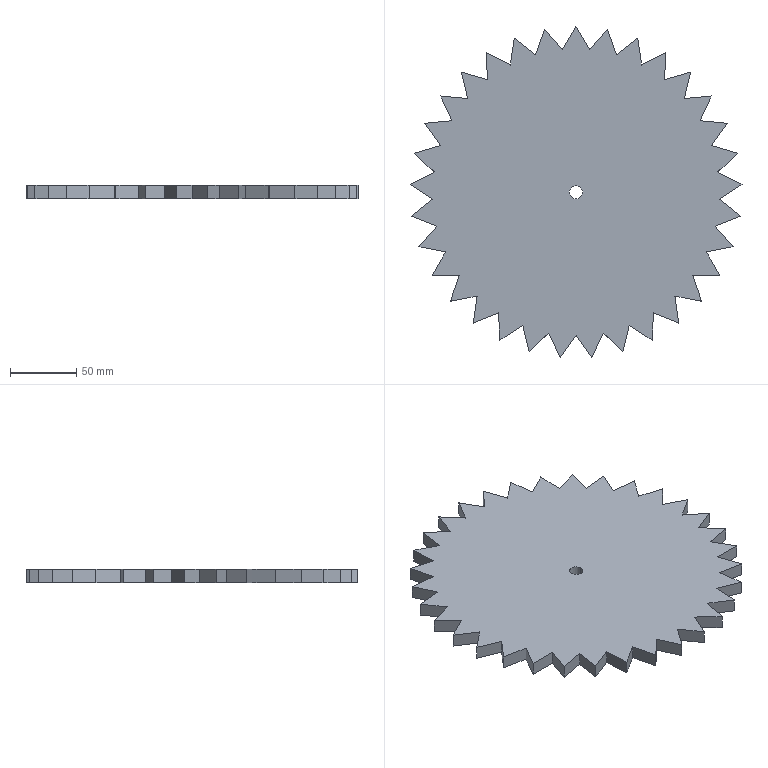Part | SolidWorks | features Extrusion 1 | 1 solid | 70 faces | box 249.717 x 249.434 x 10 mm | volume 421701 mm3 | plane 68 | cylinder 2 | commonest cylinder face diameters 10 x2